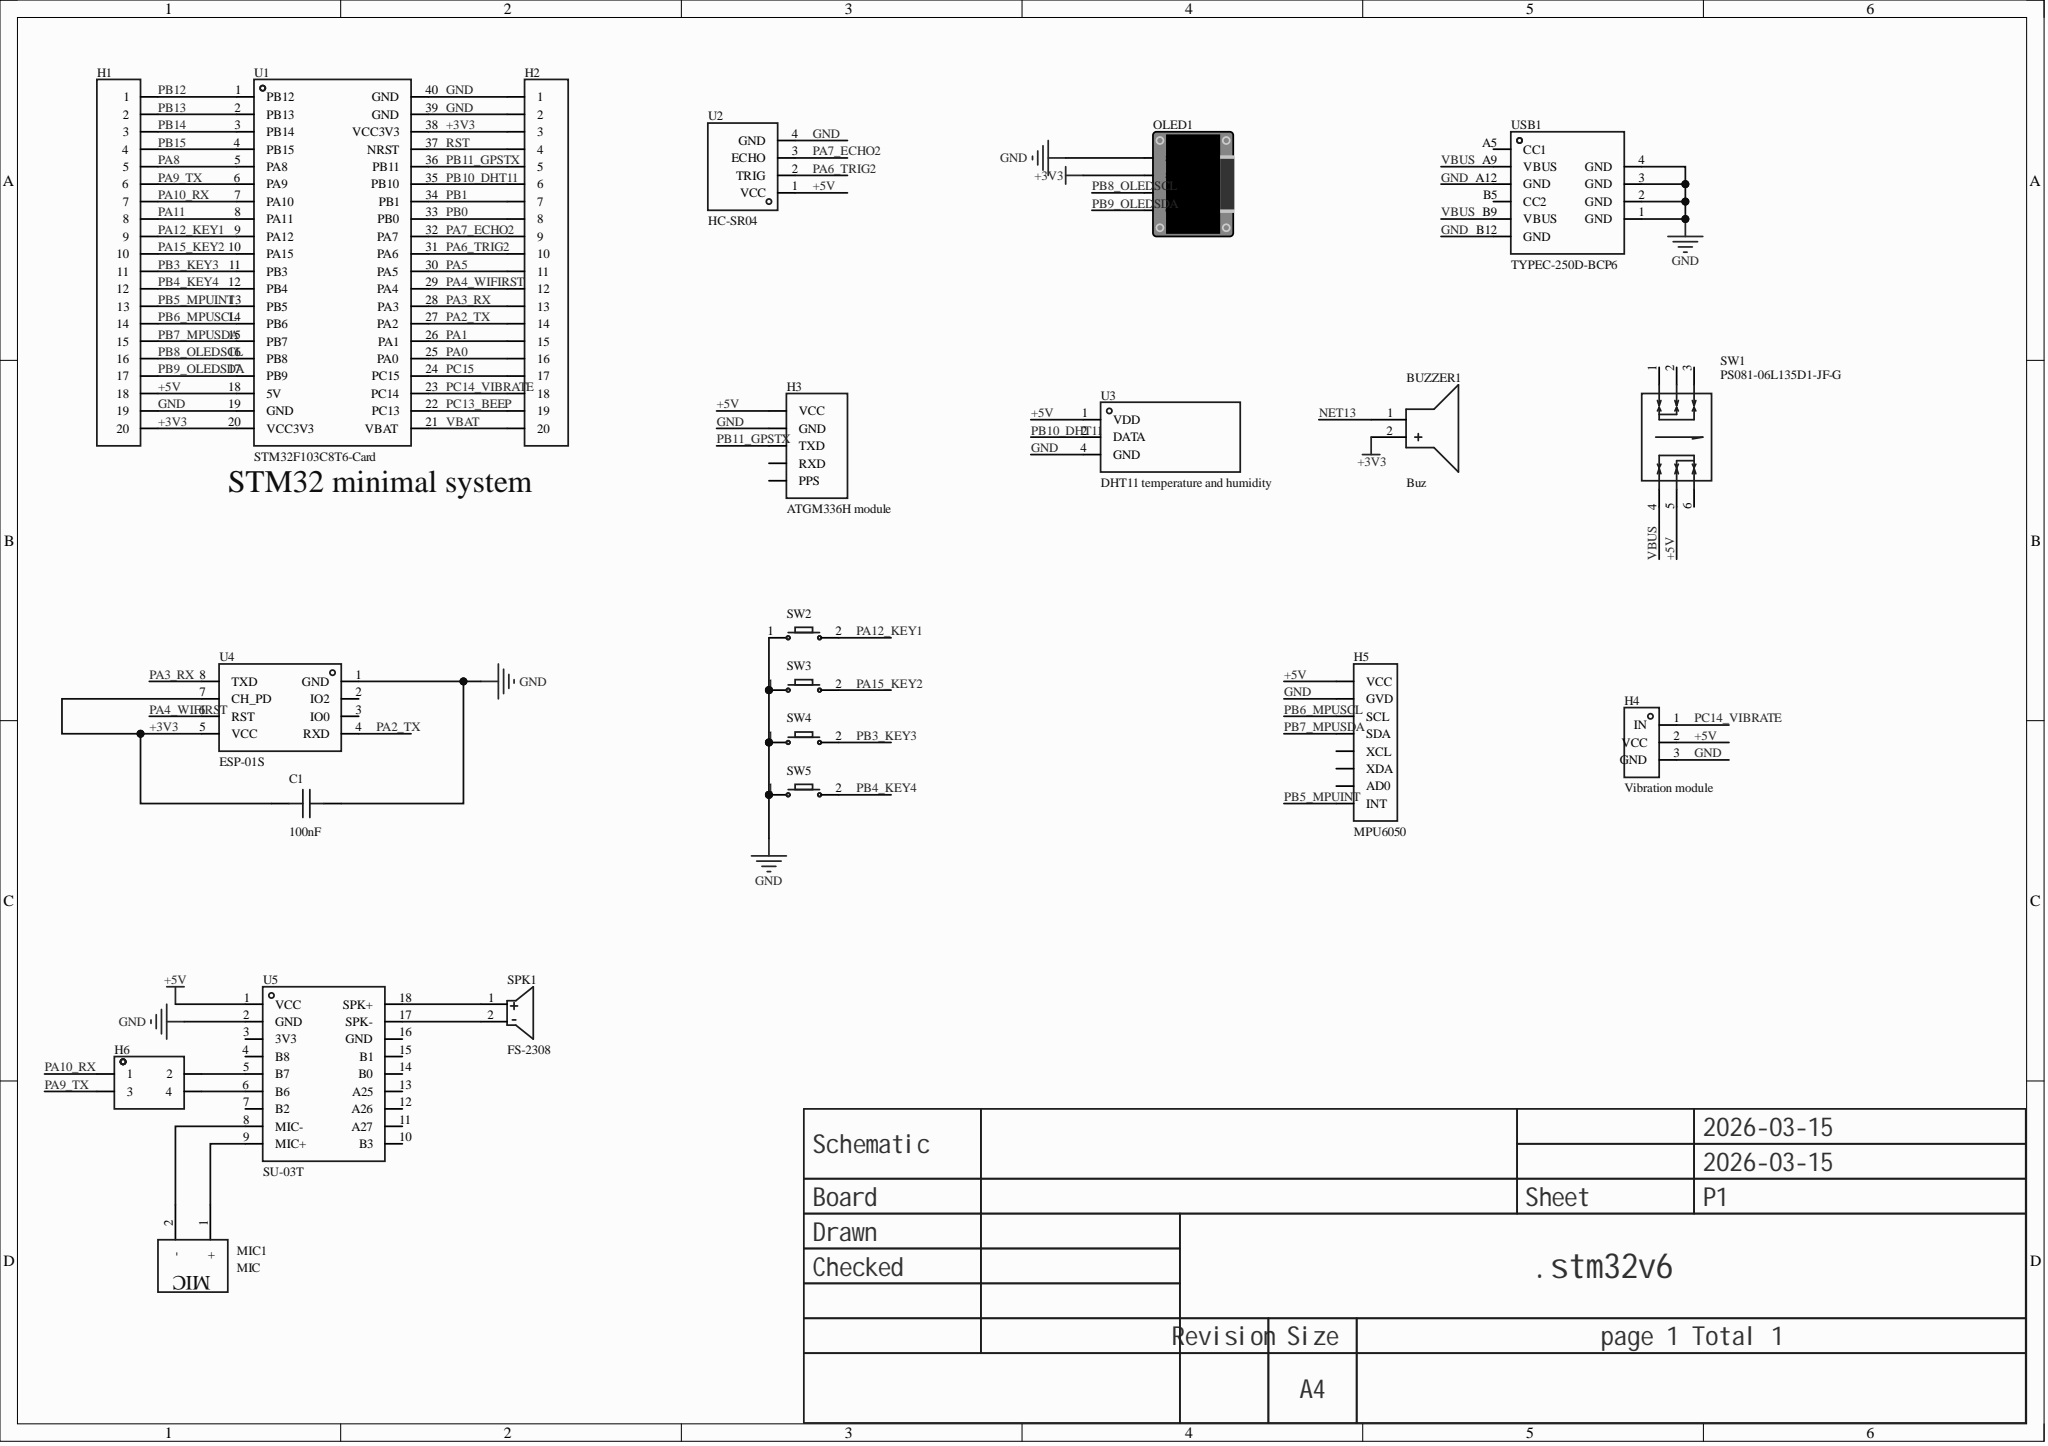Circuit board | Altium Designer | 22 parts | 44 nets
Bill of materials:
Comment,Description,Designator,Footprint,LibRef,Quantity
"Buz","","BUZZER1","BUZ-TH_BD12.0-P6.00-D0.9-RD","buzzer","1"
"100nF","","C1","C0603","CAP_0603","1"
"","","H1, H2","HDR-TH_20P-P2.54-V-F","HDR-F_2.54_1x20P","2"
"ATGM336H module","","H3","HDR-TH_5P-P2.54-V-F","HDR-F_2.54_1x5P","1"
"Vibration module","","H4","HDR-TH_3P-P2.54-V-F","HDR-F_2.54_1x3P","1"
"MPU6050","","H5","HDR-TH_8P-P2.54-V-F-1","HDR-F_2.54_1x8P","1"
"","","H6","HDR-TH_4P-P2.54-V-F-R2-C2-S2.54","HDR-F_2.54_2x2","1"
"MIC","","MIC1","MIC-TH_BD6.0-P2.00","MIC","1"
"","","OLED1","0.96OLED_4P","0.96OLED模块_4P","1"
"FS-2308","","SPK1","BEEP-TH_BD23.2-P9.20-D1.0","FS-2308","1"
"PS081-06L135D1-JF-G","8x8x13.5, 6 pcs, self-locking, black base, white XD cover, blue handle","SW1","SW-TH_6P-L8.0-W8.0-P2.50-TL","PS081-06L135D1-JF-G","1"
"","","SW2, SW3, SW4, SW5","Key_SMD_3x4x2","Key_SMD_3x4x2","4"
"STM32F103C8T6-Card","","U1","CONN-TH_L53.3-W22.9_STM32F103C8T6-CARD","STM32F103C8T6-Card","1"
"HC-SR04","","U2","TH_HC-SR04V","HC-SR04","1"
"DHT11 temperature and humidity","New capacitive digital temperature and humidity sensor; old model discontinued 16.1x12.6x5.8mm","U3","SENSOR-TH_DHT11","DHT11","1"
"ESP-01S","","U4","WIFIM-TH_ESP-01S","ESP-01S_C111009","1"
"SU-03T","Processor:-;RAM:-;USB:-;WiFi protocol:-;Bluetooth:-;Ethernet:-;","U5","COMM-SMD_18P-L21.0-W15.0-P2.00","SU-03T","1"
"TYPEC-250D-BCP6","Connector type:Type-C;Standard:USB 3.1;Gender:Female;Ports:1;Contacts:6P;Mounting:Horizontal mount;Rated current - power:3A;Operating temperature range:-25℃~+85℃;Soldering temperature (max):260℃;","USB1","USB-C-SMD_TYPEC-250D-BCP6","TYPEC-250D-BCP6","1"
Netlist (Protel format):
[
BUZZER1
BUZ-TH_BD12.0-P6.00-D0.9-RD
Buz



]
[
C1
C0603
100nF



]
[
H1
HDR-TH_20P-P2.54-V-F




]
[
H2
HDR-TH_20P-P2.54-V-F




]
[
H3
HDR-TH_5P-P2.54-V-F
ATGM336H module



]
[
H4
HDR-TH_3P-P2.54-V-F
Vibration module



]
[
H5
HDR-TH_8P-P2.54-V-F-1
MPU6050



]
[
H6
HDR-TH_4P-P2.54-V-F-R2-C2-S2.54




]
[
MIC1
MIC-TH_BD6.0-P2.00
MIC



]
[
OLED1
0.96OLED_4P




]
[
SPK1
BEEP-TH_BD23.2-P9.20-D1.0
FS-2308



]
[
SW1
SW-TH_6P-L8.0-W8.0-P2.50-TL
PS081-06L135D1-JF-G



]
[
SW2
Key_SMD_3x4x2




]
[
SW3
Key_SMD_3x4x2




]
[
SW4
Key_SMD_3x4x2




]
[
SW5
Key_SMD_3x4x2




]
[
U1
CONN-TH_L53.3-W22.9_STM32F103C8T6-CARD
STM32F103C8T6-Card



]
[
U2
TH_HC-SR04V
HC-SR04



]
[
U3
SENSOR-TH_DHT11
DHT11 temperature and humidity



]
[
U4
WIFIM-TH_ESP-01S
ESP-01S



]
[
U5
COMM-SMD_18P-L21.0-W15.0-P2.00
SU-03T



]
[
USB1
USB-C-SMD_TYPEC-250D-BCP6
TYPEC-250D-BCP6



]
(
VBUS
SW1-4
USB1-A9
USB1-B9
)
(
VBAT
H2-20
U1-21
)
(
RST
H2-4
U1-37
)
(
PC15
H2-17
U1-24
)
(
PC14_VIBRATE
H2-18
H4-1
U1-23
)
(
PC13_BEEP
H2-19
U1-22
)
(
PB15
H1-4
U1-4
)
(
PB14
H1-3
U1-3
)
(
PB13
H1-2
U1-2
)
(
PB12
H1-1
U1-1
)
(
PB11_GPSTX
H2-5
H3-3
U1-36
)
(
PB10_DHT11
H2-6
U1-35
U3-2
)
(
PB9_OLEDSDA
H1-17
OLED1-1
U1-17
)
(
PB8_OLEDSCL
H1-16
OLED1-2
U1-16
)
(
PB7_MPUSDA
H1-15
H5-4
U1-15
)
(
PB6_MPUSCL
H1-14
H5-3
U1-14
)
(
PB5_MPUINT
H1-13
H5-8
U1-13
)
(
PB4_KEY4
H1-12
SW5-2
U1-12
)
(
PB3_KEY3
H1-11
SW4-2
U1-11
)
(
PB1
H2-7
U1-34
)
(
PB0
H2-8
U1-33
)
(
PA15_KEY2
H1-10
SW3-2
U1-10
)
(
PA12_KEY1
H1-9
SW2-2
U1-9
)
(
PA11
H1-8
U1-8
)
(
PA10_RX
H1-7
H6-1
U1-7
)
(
PA9_TX
H1-6
H6-3
U1-6
)
(
PA8
H1-5
U1-5
)
(
PA7_ECHO2
H2-9
U1-32
U2-3
)
(
PA6_TRIG2
H2-10
U1-31
U2-2
)
(
PA5
H2-11
U1-30
)
(
PA4_WIFIRST
H2-12
U1-29
U4-6
)
(
PA3_RX
H2-13
U1-28
U4-8
)
(
PA2_TX
H2-14
U1-27
U4-4
)
(
PA1
H2-15
U1-26
)
(
PA0
H2-16
U1-25
)
(
NetSPK1_2
SPK1-2
U5-17
)
(
NetSPK1_1
SPK1-1
U5-18
)
(
NetMIC1_2
MIC1-2
U5-8
)
(
NetMIC1_1
MIC1-1
U5-9
)
(
NetH6_4
H6-4
U5-6
)
(
NetH6_2
H6-2
U5-5
)
(
GND
C1-2
H1-19
H2-1
H2-2
H3-2
H4-3
H5-2
OLED1-4
SW2-1
SW3-1
SW4-1
SW5-1
U1-19
U1-39
U1-40
U2-4
U3-4
U4-1
U5-2
USB1-1
USB1-2
USB1-3
USB1-4
USB1-A12
USB1-B12
)
(
+5V
H1-18
H3-1
H4-2
H5-1
SW1-5
U1-18
U2-1
U3-1
U5-1
)
(
+3V3
BUZZER1-2
C1-1
H1-20
H2-3
OLED1-3
U1-20
U1-38
U4-5
U4-7
)